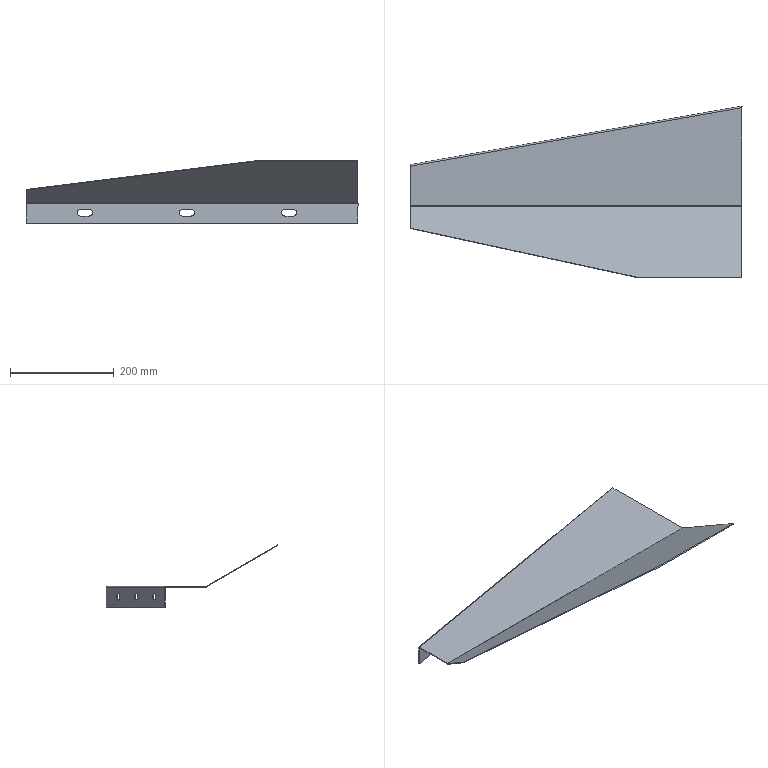Part | SolidWorks | features BaseBody 1 | 1 solid | 34 faces | box 640.37 x 331.413 x 119.799 mm | volume 282852 mm3 | plane 19 | cylinder 13 | spline 2 | commonest cylinder face diameters 13 x9 3 x2 6 x2
STEP:
#1=CARTESIAN_POINT('',(201.948,132.034,-18.5));
#2=VERTEX_POINT('',#1);
#3=CARTESIAN_POINT('',(195.547,130.905,-12.));
#4=VERTEX_POINT('',#3);
#5=CARTESIAN_POINT('',(195.547,130.905,-18.5));
#6=DIRECTION('',(0.1736,-0.9848,0.));
#7=DIRECTION('',(0.9848,0.1736,0.));
#8=AXIS2_PLACEMENT_3D('',#5,#6,#7);
#9=CIRCLE('',#8,6.5);
#10=EDGE_CURVE('',#2,#4,#9,.T.);
#11=ORIENTED_EDGE('',*,*,#10,.F.);
#12=CARTESIAN_POINT('',(202.209,130.556,-18.5));
#13=VERTEX_POINT('',#12);
#14=CARTESIAN_POINT('',(201.948,132.034,-18.5));
#15=DIRECTION('',(0.1736,-0.9848,0.));
#16=VECTOR('',#15,1000.);
#17=LINE('',#14,#16);
#18=EDGE_CURVE('',#2,#13,#17,.T.);
#19=ORIENTED_EDGE('',*,*,#18,.T.);
#20=CARTESIAN_POINT('',(195.807,129.428,-12.));
#21=VERTEX_POINT('',#20);
#22=CARTESIAN_POINT('',(195.807,129.428,-18.5));
#23=DIRECTION('',(-0.1736,0.9848,0.));
#24=DIRECTION('',(0.9848,0.1736,0.));
#25=AXIS2_PLACEMENT_3D('',#22,#23,#24);
#26=CIRCLE('',#25,6.5);
#27=EDGE_CURVE('',#21,#13,#26,.T.);
#28=ORIENTED_EDGE('',*,*,#27,.F.);
#29=CARTESIAN_POINT('',(195.807,129.428,-12.));
#30=DIRECTION('',(-0.1736,0.9848,0.));
#31=VECTOR('',#30,1000.);
#32=LINE('',#29,#31);
#33=EDGE_CURVE('',#21,#4,#32,.T.);
#34=ORIENTED_EDGE('',*,*,#33,.T.);
#35=EDGE_LOOP('',(#11,#19,#28,#34));
#36=FACE_OUTER_BOUND('',#35,.T.);
#37=CARTESIAN_POINT('',(195.547,130.905,-18.5));
#38=DIRECTION('',(0.1736,-0.9848,0.));
#39=DIRECTION('',(0.9848,0.1736,0.));
#40=AXIS2_PLACEMENT_3D('',#37,#38,#39);
#41=CYLINDRICAL_SURFACE('',#40,6.5);
#42=ADVANCED_FACE('',(#36),#41,.F.);
#43=CARTESIAN_POINT('',(-191.975,62.574,-18.5));
#44=VERTEX_POINT('',#43);
#45=CARTESIAN_POINT('',(-198.376,61.446,-12.));
#46=VERTEX_POINT('',#45);
#47=CARTESIAN_POINT('',(-198.376,61.446,-18.5));
#48=DIRECTION('',(0.1736,-0.9848,0.));
#49=DIRECTION('',(0.9848,0.1736,0.));
#50=AXIS2_PLACEMENT_3D('',#47,#48,#49);
#51=CIRCLE('',#50,6.5);
#52=EDGE_CURVE('',#44,#46,#51,.T.);
#53=ORIENTED_EDGE('',*,*,#52,.F.);
#54=CARTESIAN_POINT('',(-191.715,61.097,-18.5));
#55=VERTEX_POINT('',#54);
#56=CARTESIAN_POINT('',(-191.975,62.574,-18.5));
#57=DIRECTION('',(0.1736,-0.9848,0.));
#58=VECTOR('',#57,1000.);
#59=LINE('',#56,#58);
#60=EDGE_CURVE('',#44,#55,#59,.T.);
#61=ORIENTED_EDGE('',*,*,#60,.T.);
#62=CARTESIAN_POINT('',(-198.116,59.968,-12.));
#63=VERTEX_POINT('',#62);
#64=CARTESIAN_POINT('',(-198.116,59.968,-18.5));
#65=DIRECTION('',(-0.1736,0.9848,0.));
#66=DIRECTION('',(0.9848,0.1736,0.));
#67=AXIS2_PLACEMENT_3D('',#64,#65,#66);
#68=CIRCLE('',#67,6.5);
#69=EDGE_CURVE('',#63,#55,#68,.T.);
#70=ORIENTED_EDGE('',*,*,#69,.F.);
#71=CARTESIAN_POINT('',(-198.116,59.968,-12.));
#72=DIRECTION('',(-0.1736,0.9848,0.));
#73=VECTOR('',#72,1000.);
#74=LINE('',#71,#73);
#75=EDGE_CURVE('',#63,#46,#74,.T.);
#76=ORIENTED_EDGE('',*,*,#75,.T.);
#77=EDGE_LOOP('',(#53,#61,#70,#76));
#78=FACE_OUTER_BOUND('',#77,.T.);
#79=CARTESIAN_POINT('',(-198.376,61.446,-18.5));
#80=DIRECTION('',(0.1736,-0.9848,0.));
#81=DIRECTION('',(0.9848,0.1736,0.));
#82=AXIS2_PLACEMENT_3D('',#79,#80,#81);
#83=CYLINDRICAL_SURFACE('',#82,6.5);
#84=ADVANCED_FACE('',(#78),#83,.F.);
#85=CARTESIAN_POINT('',(4.987,97.304,-18.5));
#86=VERTEX_POINT('',#85);
#87=CARTESIAN_POINT('',(-1.415,96.175,-12.));
#88=VERTEX_POINT('',#87);
#89=CARTESIAN_POINT('',(-1.415,96.175,-18.5));
#90=DIRECTION('',(0.1736,-0.9848,0.));
#91=DIRECTION('',(0.9848,0.1736,0.));
#92=AXIS2_PLACEMENT_3D('',#89,#90,#91);
#93=CIRCLE('',#92,6.5);
#94=EDGE_CURVE('',#86,#88,#93,.T.);
#95=ORIENTED_EDGE('',*,*,#94,.F.);
#96=CARTESIAN_POINT('',(5.247,95.827,-18.5));
#97=VERTEX_POINT('',#96);
#98=CARTESIAN_POINT('',(4.987,97.304,-18.5));
#99=DIRECTION('',(0.1736,-0.9848,0.));
#100=VECTOR('',#99,1000.);
#101=LINE('',#98,#100);
#102=EDGE_CURVE('',#86,#97,#101,.T.);
#103=ORIENTED_EDGE('',*,*,#102,.T.);
#104=CARTESIAN_POINT('',(-1.154,94.698,-12.));
#105=VERTEX_POINT('',#104);
#106=CARTESIAN_POINT('',(-1.154,94.698,-18.5));
#107=DIRECTION('',(-0.1736,0.9848,0.));
#108=DIRECTION('',(0.9848,0.1736,0.));
#109=AXIS2_PLACEMENT_3D('',#106,#107,#108);
#110=CIRCLE('',#109,6.5);
#111=EDGE_CURVE('',#105,#97,#110,.T.);
#112=ORIENTED_EDGE('',*,*,#111,.F.);
#113=CARTESIAN_POINT('',(-1.154,94.698,-12.));
#114=DIRECTION('',(-0.1736,0.9848,0.));
#115=VECTOR('',#114,1000.);
#116=LINE('',#113,#115);
#117=EDGE_CURVE('',#105,#88,#116,.T.);
#118=ORIENTED_EDGE('',*,*,#117,.T.);
#119=EDGE_LOOP('',(#95,#103,#112,#118));
#120=FACE_OUTER_BOUND('',#119,.T.);
#121=CARTESIAN_POINT('',(-1.415,96.175,-18.5));
#122=DIRECTION('',(0.1736,-0.9848,0.));
#123=DIRECTION('',(0.9848,0.1736,0.));
#124=AXIS2_PLACEMENT_3D('',#121,#122,#123);
#125=CYLINDRICAL_SURFACE('',#124,6.5);
#126=ADVANCED_FACE('',(#120),#125,.F.);
#127=CARTESIAN_POINT('',(320.,149.803,1.5));
#128=VERTEX_POINT('',#127);
#129=CARTESIAN_POINT('',(-320.,36.954,1.5));
#130=VERTEX_POINT('',#129);
#131=CARTESIAN_POINT('',(320.,149.803,1.5));
#132=DIRECTION('',(-0.9848,-0.1736,0.));
#133=VECTOR('',#132,1000.);
#134=LINE('',#131,#133);
#135=EDGE_CURVE('',#128,#130,#134,.T.);
#136=ORIENTED_EDGE('',*,*,#135,.T.);
#137=CARTESIAN_POINT('',(-320.,-39.196,1.5));
#138=VERTEX_POINT('',#137);
#139=CARTESIAN_POINT('',(-320.,30.681,1.5));
#140=DIRECTION('',(0.,-1.,0.));
#141=VECTOR('',#140,1000.);
#142=LINE('',#139,#141);
#143=EDGE_CURVE('',#130,#138,#142,.T.);
#144=ORIENTED_EDGE('',*,*,#143,.T.);
#145=CARTESIAN_POINT('',(320.,-39.196,1.5));
#146=VERTEX_POINT('',#145);
#147=CARTESIAN_POINT('',(23.108,-39.196,1.5));
#148=DIRECTION('',(1.,0.,0.));
#149=VECTOR('',#148,1000.);
#150=LINE('',#147,#149);
#151=EDGE_CURVE('',#138,#146,#150,.T.);
#152=ORIENTED_EDGE('',*,*,#151,.T.);
#153=CARTESIAN_POINT('',(320.,30.681,1.5));
#154=DIRECTION('',(0.,1.,0.));
#155=VECTOR('',#154,1000.);
#156=LINE('',#153,#155);
#157=EDGE_CURVE('',#146,#128,#156,.T.);
#158=ORIENTED_EDGE('',*,*,#157,.T.);
#159=EDGE_LOOP('',(#136,#144,#152,#158));
#160=FACE_OUTER_BOUND('',#159,.T.);
#161=CARTESIAN_POINT('',(23.108,30.681,1.5));
#162=DIRECTION('',(0.,0.,1.));
#163=DIRECTION('',(1.,0.,0.));
#164=AXIS2_PLACEMENT_3D('',#161,#162,#163);
#165=PLANE('',#164);
#166=ADVANCED_FACE('',(#160),#165,.T.);
#167=CARTESIAN_POINT('',(-320.,36.954,0.));
#168=VERTEX_POINT('',#167);
#169=CARTESIAN_POINT('',(-320.,36.954,0.75));
#170=DIRECTION('',(0.,0.,1.));
#171=VECTOR('',#170,1000.);
#172=LINE('',#169,#171);
#173=EDGE_CURVE('',#168,#130,#172,.T.);
#174=ORIENTED_EDGE('',*,*,#173,.F.);
#175=CARTESIAN_POINT('',(-320.,-39.196,0.));
#176=VERTEX_POINT('',#175);
#177=CARTESIAN_POINT('',(-320.,-40.,0.));
#178=DIRECTION('',(0.,-1.,0.));
#179=VECTOR('',#178,1000.);
#180=LINE('',#177,#179);
#181=EDGE_CURVE('',#168,#176,#180,.T.);
#182=ORIENTED_EDGE('',*,*,#181,.T.);
#183=CARTESIAN_POINT('',(-320.,-40.696,0.4019));
#184=VERTEX_POINT('',#183);
#185=CARTESIAN_POINT('',(-320.,-39.196,3.));
#186=DIRECTION('',(-1.,0.,0.));
#187=DIRECTION('',(0.,-1.,0.));
#188=AXIS2_PLACEMENT_3D('',#185,#186,#187);
#189=CIRCLE('',#188,3.);
#190=EDGE_CURVE('',#176,#184,#189,.T.);
#191=ORIENTED_EDGE('',*,*,#190,.T.);
#192=CARTESIAN_POINT('',(-320.,-83.301,25.));
#193=VERTEX_POINT('',#192);
#194=CARTESIAN_POINT('',(-320.,-40.696,0.4019));
#195=DIRECTION('',(0.,-0.866,0.5));
#196=VECTOR('',#195,1000.);
#197=LINE('',#194,#196);
#198=EDGE_CURVE('',#184,#193,#197,.T.);
#199=ORIENTED_EDGE('',*,*,#198,.T.);
#200=CARTESIAN_POINT('',(-320.,-82.551,26.299));
#201=VERTEX_POINT('',#200);
#202=CARTESIAN_POINT('',(-320.,-83.301,25.));
#203=DIRECTION('',(0.,0.5,0.866));
#204=VECTOR('',#203,1000.);
#205=LINE('',#202,#204);
#206=EDGE_CURVE('',#193,#201,#205,.T.);
#207=ORIENTED_EDGE('',*,*,#206,.T.);
#208=CARTESIAN_POINT('',(-320.,-39.946,1.701));
#209=VERTEX_POINT('',#208);
#210=CARTESIAN_POINT('',(-320.,-108.39,41.217));
#211=DIRECTION('',(0.,-0.866,0.5));
#212=VECTOR('',#211,1000.);
#213=LINE('',#210,#212);
#214=EDGE_CURVE('',#209,#201,#213,.T.);
#215=ORIENTED_EDGE('',*,*,#214,.F.);
#216=CARTESIAN_POINT('',(-320.,-39.196,3.));
#217=DIRECTION('',(1.,0.,0.));
#218=DIRECTION('',(0.,-1.,0.));
#219=AXIS2_PLACEMENT_3D('',#216,#217,#218);
#220=CIRCLE('',#219,1.5);
#221=EDGE_CURVE('',#209,#138,#220,.T.);
#222=ORIENTED_EDGE('',*,*,#221,.T.);
#223=ORIENTED_EDGE('',*,*,#143,.F.);
#224=EDGE_LOOP('',(#174,#182,#191,#199,#207,#215,#222,#223));
#225=FACE_OUTER_BOUND('',#224,.T.);
#226=CARTESIAN_POINT('',(-320.,-40.,0.));
#227=DIRECTION('',(-1.,0.,0.));
#228=DIRECTION('',(0.,-1.,0.));
#229=AXIS2_PLACEMENT_3D('',#226,#227,#228);
#230=PLANE('',#229);
#231=ADVANCED_FACE('',(#225),#230,.T.);
#232=ORIENTED_EDGE('',*,*,#135,.F.);
#233=CARTESIAN_POINT('',(320.,152.849,-1.5));
#234=VERTEX_POINT('',#233);
#235=CARTESIAN_POINT('',(320.,149.803,1.5));
#236=CARTESIAN_POINT('',(319.988,150.002,1.5));
#237=CARTESIAN_POINT('',(319.975,150.198,1.481));
#238=CARTESIAN_POINT('',(319.952,150.585,1.404));
#239=CARTESIAN_POINT('',(319.94,150.777,1.346));
#240=CARTESIAN_POINT('',(319.921,151.14,1.196));
#241=CARTESIAN_POINT('',(319.912,151.314,1.104));
#242=CARTESIAN_POINT('',(319.899,151.644,0.8849));
#243=CARTESIAN_POINT('',(319.894,151.798,0.7594));
#244=CARTESIAN_POINT('',(319.89,152.078,0.4833));
#245=CARTESIAN_POINT('',(319.89,152.205,0.3309));
#246=CARTESIAN_POINT('',(319.895,152.429,0.002871));
#247=CARTESIAN_POINT('',(319.901,152.523,-0.1695));
#248=CARTESIAN_POINT('',(319.918,152.678,-0.5306));
#249=CARTESIAN_POINT('',(319.93,152.739,-0.7211));
#250=CARTESIAN_POINT('',(319.96,152.822,-1.107));
#251=CARTESIAN_POINT('',(319.978,152.845,-1.302));
#252=CARTESIAN_POINT('',(320.,152.849,-1.5));
#253=B_SPLINE_CURVE_WITH_KNOTS('',3,(#235,#236,#237,#238,#239,#240,#241,#242,#243,#244,#245,#246,#247,#248,#249,#250,#251,#252),.UNSPECIFIED.,.F.,.F.,(4,2,2,2,2,2,2,2,4),(0.,0.000592,0.001184,0.001776,0.002368,0.00296,0.003552,0.004144,0.004736),.UNSPECIFIED.);
#254=EDGE_CURVE('',#128,#234,#253,.T.);
#255=ORIENTED_EDGE('',*,*,#254,.T.);
#256=CARTESIAN_POINT('',(-320.,40.,-1.5));
#257=VERTEX_POINT('',#256);
#258=CARTESIAN_POINT('',(-0.5209,96.333,-1.5));
#259=DIRECTION('',(-0.9848,-0.1736,0.));
#260=VECTOR('',#259,1000.);
#261=LINE('',#258,#260);
#262=EDGE_CURVE('',#234,#257,#261,.T.);
#263=ORIENTED_EDGE('',*,*,#262,.T.);
#264=CARTESIAN_POINT('',(-320.,40.,-1.5));
#265=CARTESIAN_POINT('',(-320.022,39.996,-1.302));
#266=CARTESIAN_POINT('',(-320.04,39.973,-1.107));
#267=CARTESIAN_POINT('',(-320.07,39.89,-0.7214));
#268=CARTESIAN_POINT('',(-320.082,39.829,-0.5307));
#269=CARTESIAN_POINT('',(-320.099,39.674,-0.1696));
#270=CARTESIAN_POINT('',(-320.105,39.579,0.002791));
#271=CARTESIAN_POINT('',(-320.11,39.356,0.3306));
#272=CARTESIAN_POINT('',(-320.11,39.229,0.4833));
#273=CARTESIAN_POINT('',(-320.106,38.949,0.7593));
#274=CARTESIAN_POINT('',(-320.101,38.795,0.8847));
#275=CARTESIAN_POINT('',(-320.088,38.464,1.104));
#276=CARTESIAN_POINT('',(-320.079,38.291,1.196));
#277=CARTESIAN_POINT('',(-320.06,37.928,1.346));
#278=CARTESIAN_POINT('',(-320.048,37.736,1.404));
#279=CARTESIAN_POINT('',(-320.025,37.349,1.481));
#280=CARTESIAN_POINT('',(-320.012,37.153,1.5));
#281=CARTESIAN_POINT('',(-320.,36.954,1.5));
#282=B_SPLINE_CURVE_WITH_KNOTS('',3,(#264,#265,#266,#267,#268,#269,#270,#271,#272,#273,#274,#275,#276,#277,#278,#279,#280,#281),.UNSPECIFIED.,.F.,.F.,(4,2,2,2,2,2,2,2,4),(0.,0.000592,0.001184,0.001776,0.002368,0.00296,0.003552,0.004144,0.004736),.UNSPECIFIED.);
#283=EDGE_CURVE('',#257,#130,#282,.T.);
#284=ORIENTED_EDGE('',*,*,#283,.T.);
#285=EDGE_LOOP('',(#232,#255,#263,#284));
#286=FACE_OUTER_BOUND('',#285,.T.);
#287=CARTESIAN_POINT('',(0.,93.378,-1.5));
#288=DIRECTION('',(-0.9848,-0.1736,0.));
#289=DIRECTION('',(0.1736,-0.9848,0.));
#290=AXIS2_PLACEMENT_3D('',#287,#288,#289);
#291=CYLINDRICAL_SURFACE('',#290,3.);
#292=ADVANCED_FACE('',(#286),#291,.T.);
#293=CARTESIAN_POINT('',(320.,149.803,0.));
#294=VERTEX_POINT('',#293);
#295=CARTESIAN_POINT('',(320.,149.803,0.));
#296=DIRECTION('',(0.,0.,1.));
#297=VECTOR('',#296,1000.);
#298=LINE('',#295,#297);
#299=EDGE_CURVE('',#294,#128,#298,.T.);
#300=ORIENTED_EDGE('',*,*,#299,.T.);
#301=ORIENTED_EDGE('',*,*,#157,.F.);
#302=CARTESIAN_POINT('',(320.,-39.946,1.701));
#303=VERTEX_POINT('',#302);
#304=CARTESIAN_POINT('',(320.,-39.196,3.));
#305=DIRECTION('',(-1.,0.,0.));
#306=DIRECTION('',(0.,-1.,0.));
#307=AXIS2_PLACEMENT_3D('',#304,#305,#306);
#308=CIRCLE('',#307,1.5);
#309=EDGE_CURVE('',#146,#303,#308,.T.);
#310=ORIENTED_EDGE('',*,*,#309,.T.);
#311=CARTESIAN_POINT('',(320.,-177.814,81.299));
#312=VERTEX_POINT('',#311);
#313=CARTESIAN_POINT('',(320.,-108.39,41.217));
#314=DIRECTION('',(0.,0.866,-0.5));
#315=VECTOR('',#314,1000.);
#316=LINE('',#313,#315);
#317=EDGE_CURVE('',#312,#303,#316,.T.);
#318=ORIENTED_EDGE('',*,*,#317,.F.);
#319=CARTESIAN_POINT('',(320.,-178.564,80.));
#320=VERTEX_POINT('',#319);
#321=CARTESIAN_POINT('',(320.,-177.814,81.299));
#322=DIRECTION('',(0.,-0.5,-0.866));
#323=VECTOR('',#322,1000.);
#324=LINE('',#321,#323);
#325=EDGE_CURVE('',#312,#320,#324,.T.);
#326=ORIENTED_EDGE('',*,*,#325,.T.);
#327=CARTESIAN_POINT('',(320.,-40.696,0.4019));
#328=VERTEX_POINT('',#327);
#329=CARTESIAN_POINT('',(320.,-178.564,80.));
#330=DIRECTION('',(0.,0.866,-0.5));
#331=VECTOR('',#330,1000.);
#332=LINE('',#329,#331);
#333=EDGE_CURVE('',#320,#328,#332,.T.);
#334=ORIENTED_EDGE('',*,*,#333,.T.);
#335=CARTESIAN_POINT('',(320.,-39.196,0.));
#336=VERTEX_POINT('',#335);
#337=CARTESIAN_POINT('',(320.,-39.196,3.));
#338=DIRECTION('',(1.,0.,0.));
#339=DIRECTION('',(0.,-1.,0.));
#340=AXIS2_PLACEMENT_3D('',#337,#338,#339);
#341=CIRCLE('',#340,3.);
#342=EDGE_CURVE('',#328,#336,#341,.T.);
#343=ORIENTED_EDGE('',*,*,#342,.T.);
#344=CARTESIAN_POINT('',(320.,40.,0.));
#345=DIRECTION('',(0.,1.,0.));
#346=VECTOR('',#345,1000.);
#347=LINE('',#344,#346);
#348=EDGE_CURVE('',#336,#294,#347,.T.);
#349=ORIENTED_EDGE('',*,*,#348,.T.);
#350=EDGE_LOOP('',(#300,#301,#310,#318,#326,#334,#343,#349));
#351=FACE_OUTER_BOUND('',#350,.T.);
#352=CARTESIAN_POINT('',(320.,40.,0.));
#353=DIRECTION('',(1.,0.,0.));
#354=DIRECTION('',(0.,0.,-1.));
#355=AXIS2_PLACEMENT_3D('',#352,#353,#354);
#356=PLANE('',#355);
#357=ADVANCED_FACE('',(#351),#356,.T.);
#358=ORIENTED_EDGE('',*,*,#309,.F.);
#359=ORIENTED_EDGE('',*,*,#151,.F.);
#360=ORIENTED_EDGE('',*,*,#221,.F.);
#361=CARTESIAN_POINT('',(0.,-39.946,1.701));
#362=DIRECTION('',(-1.,0.,0.));
#363=VECTOR('',#362,1000.);
#364=LINE('',#361,#363);
#365=EDGE_CURVE('',#303,#209,#364,.T.);
#366=ORIENTED_EDGE('',*,*,#365,.F.);
#367=EDGE_LOOP('',(#358,#359,#360,#366));
#368=FACE_OUTER_BOUND('',#367,.T.);
#369=CARTESIAN_POINT('',(0.,-39.196,3.));
#370=DIRECTION('',(-1.,0.,0.));
#371=DIRECTION('',(0.,-1.,0.));
#372=AXIS2_PLACEMENT_3D('',#369,#370,#371);
#373=CYLINDRICAL_SURFACE('',#372,1.5);
#374=ADVANCED_FACE('',(#368),#373,.F.);
#375=ORIENTED_EDGE('',*,*,#181,.F.);
#376=CARTESIAN_POINT('',(320.,149.803,0.));
#377=DIRECTION('',(-0.9848,-0.1736,0.));
#378=VECTOR('',#377,1000.);
#379=LINE('',#376,#378);
#380=EDGE_CURVE('',#294,#168,#379,.T.);
#381=ORIENTED_EDGE('',*,*,#380,.F.);
#382=ORIENTED_EDGE('',*,*,#348,.F.);
#383=CARTESIAN_POINT('',(23.108,-39.196,0.));
#384=DIRECTION('',(1.,0.,0.));
#385=VECTOR('',#384,1000.);
#386=LINE('',#383,#385);
#387=EDGE_CURVE('',#176,#336,#386,.T.);
#388=ORIENTED_EDGE('',*,*,#387,.F.);
#389=EDGE_LOOP('',(#375,#381,#382,#388));
#390=FACE_OUTER_BOUND('',#389,.T.);
#391=CARTESIAN_POINT('',(23.108,30.681,0.));
#392=DIRECTION('',(0.,0.,1.));
#393=DIRECTION('',(1.,0.,0.));
#394=AXIS2_PLACEMENT_3D('',#391,#392,#393);
#395=PLANE('',#394);
#396=ADVANCED_FACE('',(#390),#395,.F.);
#397=CARTESIAN_POINT('',(320.26,151.372,-1.5));
#398=VERTEX_POINT('',#397);
#399=CARTESIAN_POINT('',(320.,149.803,0.));
#400=CARTESIAN_POINT('',(320.009,150.006,0.));
#401=CARTESIAN_POINT('',(320.019,150.205,-0.03888));
#402=CARTESIAN_POINT('',(320.036,150.485,-0.1518));
#403=CARTESIAN_POINT('',(320.043,150.573,-0.1979));
#404=CARTESIAN_POINT('',(320.058,150.741,-0.3065));
#405=CARTESIAN_POINT('',(320.067,150.821,-0.3698));
#406=CARTESIAN_POINT('',(320.086,150.965,-0.5082));
#407=CARTESIAN_POINT('',(320.097,151.03,-0.5836));
#408=CARTESIAN_POINT('',(320.121,151.145,-0.7469));
#409=CARTESIAN_POINT('',(320.135,151.195,-0.8347));
#410=CARTESIAN_POINT('',(320.18,151.318,-1.105));
#411=CARTESIAN_POINT('',(320.217,151.364,-1.302));
#412=CARTESIAN_POINT('',(320.26,151.372,-1.5));
#413=B_SPLINE_CURVE_WITH_KNOTS('',3,(#399,#400,#401,#402,#403,#404,#405,#406,#407,#408,#409,#410,#411,#412),.UNSPECIFIED.,.F.,.F.,(4,2,2,2,2,2,4),(0.,0.0006004,0.0009005,0.001201,0.001501,0.001801,0.002401),.UNSPECIFIED.);
#414=EDGE_CURVE('',#294,#398,#413,.T.);
#415=ORIENTED_EDGE('',*,*,#414,.T.);
#416=CARTESIAN_POINT('',(320.26,151.372,-1.5));
#417=DIRECTION('',(0.1736,-0.9848,0.));
#418=VECTOR('',#417,1000.);
#419=LINE('',#416,#418);
#420=EDGE_CURVE('',#234,#398,#419,.T.);
#421=ORIENTED_EDGE('',*,*,#420,.F.);
#422=ORIENTED_EDGE('',*,*,#254,.F.);
#423=ORIENTED_EDGE('',*,*,#299,.F.);
#424=EDGE_LOOP('',(#415,#421,#422,#423));
#425=FACE_OUTER_BOUND('',#424,.T.);
#426=CARTESIAN_POINT('',(320.,149.803,1.516));
#427=CARTESIAN_POINT('',(319.957,150.483,1.516));
#428=CARTESIAN_POINT('',(319.856,152.07,0.9637));
#429=CARTESIAN_POINT('',(319.898,152.847,-0.5977));
#430=CARTESIAN_POINT('',(319.997,152.865,-1.5));
#431=CARTESIAN_POINT('',(320.,149.803,1.511));
#432=CARTESIAN_POINT('',(319.957,150.481,1.511));
#433=CARTESIAN_POINT('',(319.857,152.066,0.9594));
#434=CARTESIAN_POINT('',(319.899,152.842,-0.5993));
#435=CARTESIAN_POINT('',(319.998,152.86,-1.5));
#436=CARTESIAN_POINT('',(320.,149.803,1.505));
#437=CARTESIAN_POINT('',(319.957,150.48,1.505));
#438=CARTESIAN_POINT('',(319.857,152.062,0.9551));
#439=CARTESIAN_POINT('',(319.9,152.837,-0.6008));
#440=CARTESIAN_POINT('',(319.999,152.854,-1.5));
#441=CARTESIAN_POINT('',(320.,149.803,1.5));
#442=CARTESIAN_POINT('',(319.958,150.479,1.5));
#443=CARTESIAN_POINT('',(319.858,152.059,0.9508));
#444=CARTESIAN_POINT('',(319.901,152.832,-0.6024));
#445=CARTESIAN_POINT('',(320.,152.849,-1.5));
#446=CARTESIAN_POINT('',(320.,149.803,1.));
#447=CARTESIAN_POINT('',(319.977,150.369,1.));
#448=CARTESIAN_POINT('',(319.923,151.69,0.5423));
#449=CARTESIAN_POINT('',(319.988,152.339,-0.752));
#450=CARTESIAN_POINT('',(320.087,152.357,-1.5));
#451=CARTESIAN_POINT('',(320.,149.803,0.5));
#452=CARTESIAN_POINT('',(319.996,150.258,0.5));
#453=CARTESIAN_POINT('',(319.988,151.321,0.1339));
#454=CARTESIAN_POINT('',(320.074,151.847,-0.9016));
#455=CARTESIAN_POINT('',(320.174,151.864,-1.5));
#456=CARTESIAN_POINT('',(320.,149.803,0.));
#457=CARTESIAN_POINT('',(320.016,150.148,0.));
#458=CARTESIAN_POINT('',(320.053,150.953,-0.2746));
#459=CARTESIAN_POINT('',(320.161,151.355,-1.051));
#460=CARTESIAN_POINT('',(320.26,151.372,-1.5));
#461=CARTESIAN_POINT('',(320.,149.803,-0.005053));
#462=CARTESIAN_POINT('',(320.016,150.146,-0.005053));
#463=CARTESIAN_POINT('',(320.054,150.949,-0.2787));
#464=CARTESIAN_POINT('',(320.162,151.35,-1.053));
#465=CARTESIAN_POINT('',(320.261,151.367,-1.5));
#466=CARTESIAN_POINT('',(320.,149.803,-0.01011));
#467=CARTESIAN_POINT('',(320.016,150.145,-0.01011));
#468=CARTESIAN_POINT('',(320.054,150.945,-0.2829));
#469=CARTESIAN_POINT('',(320.163,151.345,-1.054));
#470=CARTESIAN_POINT('',(320.262,151.362,-1.5));
#471=CARTESIAN_POINT('',(320.,149.803,-0.01516));
#472=CARTESIAN_POINT('',(320.017,150.144,-0.01516));
#473=CARTESIAN_POINT('',(320.055,150.941,-0.287));
#474=CARTESIAN_POINT('',(320.164,151.34,-1.056));
#475=CARTESIAN_POINT('',(320.263,151.357,-1.5));
#476=B_SPLINE_SURFACE_WITH_KNOTS('',3,3,((#426,#427,#428,#429,#430),(#431,#432,#433,#434,#435),(#436,#437,#438,#439,#440),(#441,#442,#443,#444,#445),(#446,#447,#448,#449,#450),(#451,#452,#453,#454,#455),(#456,#457,#458,#459,#460),(#461,#462,#463,#464,#465),(#466,#467,#468,#469,#470),(#471,#472,#473,#474,#475)),.UNSPECIFIED.,.F.,.F.,.F.,(4,3,3,4),(4,1,4),(-0.1516,-0.15,0.,0.001516),(-0.3434,-0.1962,0.),.UNSPECIFIED.);
#477=ADVANCED_FACE('',(#425),#476,.T.);
#478=CARTESIAN_POINT('',(-319.74,38.523,-1.5));
#479=VERTEX_POINT('',#478);
#480=CARTESIAN_POINT('',(-319.74,38.523,-1.5));
#481=CARTESIAN_POINT('',(-319.783,38.515,-1.302));
#482=CARTESIAN_POINT('',(-319.82,38.469,-1.108));
#483=CARTESIAN_POINT('',(-319.865,38.346,-0.8351));
#484=CARTESIAN_POINT('',(-319.879,38.297,-0.749));
#485=CARTESIAN_POINT('',(-319.903,38.183,-0.5862));
#486=CARTESIAN_POINT('',(-319.914,38.117,-0.5089));
#487=CARTESIAN_POINT('',(-319.933,37.973,-0.3704));
#488=CARTESIAN_POINT('',(-319.942,37.894,-0.3084));
#489=CARTESIAN_POINT('',(-319.957,37.726,-0.199));
#490=CARTESIAN_POINT('',(-319.964,37.636,-0.1521));
#491=CARTESIAN_POINT('',(-319.981,37.358,-0.03974));
#492=CARTESIAN_POINT('',(-319.991,37.157,0.));
#493=CARTESIAN_POINT('',(-320.,36.954,0.));
#494=B_SPLINE_CURVE_WITH_KNOTS('',3,(#480,#481,#482,#483,#484,#485,#486,#487,#488,#489,#490,#491,#492,#493),.UNSPECIFIED.,.F.,.F.,(4,2,2,2,2,2,4),(0.,0.0006004,0.0009006,0.001201,0.001501,0.001801,0.002401),.UNSPECIFIED.);
#495=EDGE_CURVE('',#479,#168,#494,.T.);
#496=ORIENTED_EDGE('',*,*,#495,.T.);
#497=ORIENTED_EDGE('',*,*,#173,.T.);
#498=ORIENTED_EDGE('',*,*,#283,.F.);
#499=CARTESIAN_POINT('',(-319.74,38.523,-1.5));
#500=DIRECTION('',(-0.1736,0.9848,0.));
#501=VECTOR('',#500,1000.);
#502=LINE('',#499,#501);
#503=EDGE_CURVE('',#479,#257,#502,.T.);
#504=ORIENTED_EDGE('',*,*,#503,.F.);
#505=EDGE_LOOP('',(#496,#497,#498,#504));
#506=FACE_OUTER_BOUND('',#505,.T.);
#507=CARTESIAN_POINT('',(-320.,36.954,-0.01516));
#508=CARTESIAN_POINT('',(-319.983,37.295,-0.01516));
#509=CARTESIAN_POINT('',(-319.945,38.092,-0.287));
#510=CARTESIAN_POINT('',(-319.836,38.49,-1.056));
#511=CARTESIAN_POINT('',(-319.737,38.508,-1.5));
#512=CARTESIAN_POINT('',(-320.,36.954,-0.0101));
#513=CARTESIAN_POINT('',(-319.984,37.296,-0.0101));
#514=CARTESIAN_POINT('',(-319.946,38.096,-0.2828));
#515=CARTESIAN_POINT('',(-319.837,38.495,-1.054));
#516=CARTESIAN_POINT('',(-319.738,38.513,-1.5));
#517=CARTESIAN_POINT('',(-320.,36.954,-0.005052));
#518=CARTESIAN_POINT('',(-319.984,37.297,-0.005052));
#519=CARTESIAN_POINT('',(-319.946,38.1,-0.2787));
#520=CARTESIAN_POINT('',(-319.838,38.5,-1.053));
#521=CARTESIAN_POINT('',(-319.739,38.518,-1.5));
#522=CARTESIAN_POINT('',(-320.,36.954,0.));
#523=CARTESIAN_POINT('',(-319.984,37.298,0.));
#524=CARTESIAN_POINT('',(-319.947,38.103,-0.2746));
#525=CARTESIAN_POINT('',(-319.839,38.505,-1.051));
#526=CARTESIAN_POINT('',(-319.74,38.523,-1.5));
#527=CARTESIAN_POINT('',(-320.,36.954,0.5));
#528=CARTESIAN_POINT('',(-320.004,37.409,0.5));
#529=CARTESIAN_POINT('',(-320.012,38.472,0.1339));
#530=CARTESIAN_POINT('',(-319.926,38.998,-0.9016));
#531=CARTESIAN_POINT('',(-319.826,39.015,-1.5));
#532=CARTESIAN_POINT('',(-320.,36.954,1.));
#533=CARTESIAN_POINT('',(-320.023,37.519,1.));
#534=CARTESIAN_POINT('',(-320.077,38.841,0.5423));
#535=CARTESIAN_POINT('',(-320.012,39.49,-0.752));
#536=CARTESIAN_POINT('',(-319.913,39.508,-1.5));
#537=CARTESIAN_POINT('',(-320.,36.954,1.5));
#538=CARTESIAN_POINT('',(-320.042,37.63,1.5));
#539=CARTESIAN_POINT('',(-320.142,39.209,0.9508));
#540=CARTESIAN_POINT('',(-320.099,39.983,-0.6024));
#541=CARTESIAN_POINT('',(-320.,40.,-1.5));
#542=CARTESIAN_POINT('',(-320.,36.954,1.505));
#543=CARTESIAN_POINT('',(-320.043,37.631,1.505));
#544=CARTESIAN_POINT('',(-320.143,39.213,0.9551));
#545=CARTESIAN_POINT('',(-320.1,39.988,-0.6008));
#546=CARTESIAN_POINT('',(-320.001,40.005,-1.5));
#547=CARTESIAN_POINT('',(-320.,36.954,1.51));
#548=CARTESIAN_POINT('',(-320.043,37.632,1.51));
#549=CARTESIAN_POINT('',(-320.143,39.217,0.9594));
#550=CARTESIAN_POINT('',(-320.101,39.993,-0.5993));
#551=CARTESIAN_POINT('',(-320.002,40.01,-1.5));
#552=CARTESIAN_POINT('',(-320.,36.954,1.516));
#553=CARTESIAN_POINT('',(-320.043,37.633,1.516));
#554=CARTESIAN_POINT('',(-320.144,39.221,0.9637));
#555=CARTESIAN_POINT('',(-320.102,39.998,-0.5977));
#556=CARTESIAN_POINT('',(-320.003,40.016,-1.5));
#557=B_SPLINE_SURFACE_WITH_KNOTS('',3,3,((#507,#508,#509,#510,#511),(#512,#513,#514,#515,#516),(#517,#518,#519,#520,#521),(#522,#523,#524,#525,#526),(#527,#528,#529,#530,#531),(#532,#533,#534,#535,#536),(#537,#538,#539,#540,#541),(#542,#543,#544,#545,#546),(#547,#548,#549,#550,#551),(#552,#553,#554,#555,#556)),.UNSPECIFIED.,.F.,.F.,.F.,(4,3,3,4),(4,1,4),(-0.001516,0.,0.15,0.1516),(0.,0.1472,0.3434),.UNSPECIFIED.);
#558=ADVANCED_FACE('',(#506),#557,.T.);
#559=CARTESIAN_POINT('',(178.805,127.953,-12.));
#560=VERTEX_POINT('',#559);
#561=CARTESIAN_POINT('',(178.805,127.953,-25.));
#562=VERTEX_POINT('',#561);
#563=CARTESIAN_POINT('',(178.805,127.953,-18.5));
#564=DIRECTION('',(0.1736,-0.9848,0.));
#565=DIRECTION('',(0.9848,0.1736,0.));
#566=AXIS2_PLACEMENT_3D('',#563,#564,#565);
#567=CIRCLE('',#566,6.5);
#568=EDGE_CURVE('',#560,#562,#567,.T.);
#569=ORIENTED_EDGE('',*,*,#568,.T.);
#570=CARTESIAN_POINT('',(195.547,130.905,-25.));
#571=VERTEX_POINT('',#570);
#572=CARTESIAN_POINT('',(-0.2465,96.381,-25.));
#573=DIRECTION('',(0.9848,0.1736,0.));
#574=VECTOR('',#573,1000.);
#575=LINE('',#572,#574);
#576=EDGE_CURVE('',#562,#571,#575,.T.);
#577=ORIENTED_EDGE('',*,*,#576,.T.);
#578=CARTESIAN_POINT('',(195.547,130.905,-18.5));
#579=DIRECTION('',(0.1736,-0.9848,0.));
#580=DIRECTION('',(0.9848,0.1736,0.));
#581=AXIS2_PLACEMENT_3D('',#578,#579,#580);
#582=CIRCLE('',#581,6.5);
#583=EDGE_CURVE('',#571,#2,#582,.T.);
#584=ORIENTED_EDGE('',*,*,#583,.T.);
#585=ORIENTED_EDGE('',*,*,#10,.T.);
#586=CARTESIAN_POINT('',(-0.2465,96.381,-12.));
#587=DIRECTION('',(-0.9848,-0.1736,0.));
#588=VECTOR('',#587,1000.);
#589=LINE('',#586,#588);
#590=EDGE_CURVE('',#4,#560,#589,.T.);
#591=ORIENTED_EDGE('',*,*,#590,.T.);
#592=EDGE_LOOP('',(#569,#577,#584,#585,#591));
#593=FACE_BOUND('',#592,.T.);
#594=CARTESIAN_POINT('',(-215.118,58.494,-12.));
#595=VERTEX_POINT('',#594);
#596=CARTESIAN_POINT('',(-215.118,58.494,-25.));
#597=VERTEX_POINT('',#596);
#598=CARTESIAN_POINT('',(-215.118,58.494,-18.5));
#599=DIRECTION('',(0.1736,-0.9848,0.));
#600=DIRECTION('',(0.9848,0.1736,0.));
#601=AXIS2_PLACEMENT_3D('',#598,#599,#600);
#602=CIRCLE('',#601,6.5);
#603=EDGE_CURVE('',#595,#597,#602,.T.);
#604=ORIENTED_EDGE('',*,*,#603,.T.);
#605=CARTESIAN_POINT('',(-198.376,61.446,-25.));
#606=VERTEX_POINT('',#605);
#607=CARTESIAN_POINT('',(-0.2465,96.381,-25.));
#608=DIRECTION('',(0.9848,0.1736,0.));
#609=VECTOR('',#608,1000.);
#610=LINE('',#607,#609);
#611=EDGE_CURVE('',#597,#606,#610,.T.);
#612=ORIENTED_EDGE('',*,*,#611,.T.);
#613=CARTESIAN_POINT('',(-198.376,61.446,-18.5));
#614=DIRECTION('',(0.1736,-0.9848,0.));
#615=DIRECTION('',(0.9848,0.1736,0.));
#616=AXIS2_PLACEMENT_3D('',#613,#614,#615);
#617=CIRCLE('',#616,6.5);
#618=EDGE_CURVE('',#606,#44,#617,.T.);
#619=ORIENTED_EDGE('',*,*,#618,.T.);
#620=ORIENTED_EDGE('',*,*,#52,.T.);
#621=CARTESIAN_POINT('',(-0.2465,96.381,-12.));
#622=DIRECTION('',(-0.9848,-0.1736,0.));
#623=VECTOR('',#622,1000.);
#624=LINE('',#621,#623);
#625=EDGE_CURVE('',#46,#595,#624,.T.);
#626=ORIENTED_EDGE('',*,*,#625,.T.);
#627=EDGE_LOOP('',(#604,#612,#619,#620,#626));
#628=FACE_BOUND('',#627,.T.);
#629=CARTESIAN_POINT('',(-18.156,93.223,-12.));
#630=VERTEX_POINT('',#629);
#631=CARTESIAN_POINT('',(-18.156,93.223,-25.));
#632=VERTEX_POINT('',#631);
#633=CARTESIAN_POINT('',(-18.156,93.223,-18.5));
#634=DIRECTION('',(0.1736,-0.9848,0.));
#635=DIRECTION('',(0.9848,0.1736,0.));
#636=AXIS2_PLACEMENT_3D('',#633,#634,#635);
#637=CIRCLE('',#636,6.5);
#638=EDGE_CURVE('',#630,#632,#637,.T.);
#639=ORIENTED_EDGE('',*,*,#638,.T.);
#640=CARTESIAN_POINT('',(-1.415,96.175,-25.));
#641=VERTEX_POINT('',#640);
#642=CARTESIAN_POINT('',(-0.2465,96.381,-25.));
#643=DIRECTION('',(0.9848,0.1736,0.));
#644=VECTOR('',#643,1000.);
#645=LINE('',#642,#644);
#646=EDGE_CURVE('',#632,#641,#645,.T.);
#647=ORIENTED_EDGE('',*,*,#646,.T.);
#648=CARTESIAN_POINT('',(-1.415,96.175,-18.5));
#649=DIRECTION('',(0.1736,-0.9848,0.));
#650=DIRECTION('',(0.9848,0.1736,0.));
#651=AXIS2_PLACEMENT_3D('',#648,#649,#650);
#652=CIRCLE('',#651,6.5);
#653=EDGE_CURVE('',#641,#86,#652,.T.);
#654=ORIENTED_EDGE('',*,*,#653,.T.);
#655=ORIENTED_EDGE('',*,*,#94,.T.);
#656=CARTESIAN_POINT('',(-0.2465,96.381,-12.));
#657=DIRECTION('',(-0.9848,-0.1736,0.));
#658=VECTOR('',#657,1000.);
#659=LINE('',#656,#658);
#660=EDGE_CURVE('',#88,#630,#659,.T.);
#661=ORIENTED_EDGE('',*,*,#660,.T.);
#662=EDGE_LOOP('',(#639,#647,#654,#655,#661));
#663=FACE_BOUND('',#662,.T.);
#664=CARTESIAN_POINT('',(320.,152.849,-38.5));
#665=VERTEX_POINT('',#664);
#666=CARTESIAN_POINT('',(-320.,40.,-38.5));
#667=VERTEX_POINT('',#666);
#668=CARTESIAN_POINT('',(-0.2465,96.381,-38.5));
#669=DIRECTION('',(-0.9848,-0.1736,0.));
#670=VECTOR('',#669,1000.);
#671=LINE('',#668,#670);
#672=EDGE_CURVE('',#665,#667,#671,.T.);
#673=ORIENTED_EDGE('',*,*,#672,.T.);
#674=CARTESIAN_POINT('',(-320.,40.,-18.302));
#675=DIRECTION('',(0.,0.,1.));
#676=VECTOR('',#675,1000.);
#677=LINE('',#674,#676);
#678=EDGE_CURVE('',#667,#257,#677,.T.);
#679=ORIENTED_EDGE('',*,*,#678,.T.);
#680=ORIENTED_EDGE('',*,*,#262,.F.);
#681=CARTESIAN_POINT('',(320.,152.849,-18.302));
#682=DIRECTION('',(0.,0.,-1.));
#683=VECTOR('',#682,1000.);
#684=LINE('',#681,#683);
#685=EDGE_CURVE('',#234,#665,#684,.T.);
#686=ORIENTED_EDGE('',*,*,#685,.T.);
#687=EDGE_LOOP('',(#673,#679,#680,#686));
#688=FACE_OUTER_BOUND('',#687,.T.);
#689=CARTESIAN_POINT('',(-0.2465,96.381,-18.302));
#690=DIRECTION('',(-0.1736,0.9848,0.));
#691=DIRECTION('',(-0.9848,-0.1736,0.));
#692=AXIS2_PLACEMENT_3D('',#689,#690,#691);
#693=PLANE('',#692);
#694=ADVANCED_FACE('',(#593,#628,#663,#688),#693,.T.);
#695=ORIENTED_EDGE('',*,*,#365,.T.);
#696=ORIENTED_EDGE('',*,*,#214,.T.);
#697=CARTESIAN_POINT('',(120.,-177.814,81.299));
#698=VERTEX_POINT('',#697);
#699=CARTESIAN_POINT('',(-320.,-82.551,26.299));
#700=DIRECTION('',(0.9701,-0.21,0.1213));
#701=VECTOR('',#700,1000.);
#702=LINE('',#699,#701);
#703=EDGE_CURVE('',#201,#698,#702,.T.);
#704=ORIENTED_EDGE('',*,*,#703,.T.);
#705=CARTESIAN_POINT('',(0.,-177.814,81.299));
#706=DIRECTION('',(1.,0.,0.));
#707=VECTOR('',#706,1000.);
#708=LINE('',#705,#707);
#709=EDGE_CURVE('',#698,#312,#708,.T.);
#710=ORIENTED_EDGE('',*,*,#709,.T.);
#711=ORIENTED_EDGE('',*,*,#317,.T.);
#712=EDGE_LOOP('',(#695,#696,#704,#710,#711));
#713=FACE_OUTER_BOUND('',#712,.T.);
#714=CARTESIAN_POINT('',(0.,-108.39,41.217));
#715=DIRECTION('',(0.,0.5,0.866));
#716=DIRECTION('',(0.,-0.866,0.5));
#717=AXIS2_PLACEMENT_3D('',#714,#715,#716);
#718=PLANE('',#717);
#719=ADVANCED_FACE('',(#713),#718,.T.);
#720=ORIENTED_EDGE('',*,*,#387,.T.);
#721=ORIENTED_EDGE('',*,*,#342,.F.);
#722=CARTESIAN_POINT('',(0.,-40.696,0.4019));
#723=DIRECTION('',(-1.,0.,0.));
#724=VECTOR('',#723,1000.);
#725=LINE('',#722,#724);
#726=EDGE_CURVE('',#328,#184,#725,.T.);
#727=ORIENTED_EDGE('',*,*,#726,.T.);
#728=ORIENTED_EDGE('',*,*,#190,.F.);
#729=EDGE_LOOP('',(#720,#721,#727,#728));
#730=FACE_OUTER_BOUND('',#729,.T.);
#731=CARTESIAN_POINT('',(0.,-39.196,3.));
#732=DIRECTION('',(-1.,0.,0.));
#733=DIRECTION('',(0.,-1.,0.));
#734=AXIS2_PLACEMENT_3D('',#731,#732,#733);
#735=CYLINDRICAL_SURFACE('',#734,3.);
#736=ADVANCED_FACE('',(#730),#735,.T.);
#737=ORIENTED_EDGE('',*,*,#414,.F.);
#738=ORIENTED_EDGE('',*,*,#380,.T.);
#739=ORIENTED_EDGE('',*,*,#495,.F.);
#740=CARTESIAN_POINT('',(-0.2605,94.856,-1.5));
#741=DIRECTION('',(-0.9848,-0.1736,0.));
#742=VECTOR('',#741,1000.);
#743=LINE('',#740,#742);
#744=EDGE_CURVE('',#398,#479,#743,.T.);
#745=ORIENTED_EDGE('',*,*,#744,.F.);
#746=EDGE_LOOP('',(#737,#738,#739,#745));
#747=FACE_OUTER_BOUND('',#746,.T.);
#748=CARTESIAN_POINT('',(0.,93.378,-1.5));
#749=DIRECTION('',(-0.9848,-0.1736,0.));
#750=DIRECTION('',(0.1736,-0.9848,0.));
#751=AXIS2_PLACEMENT_3D('',#748,#749,#750);
#752=CYLINDRICAL_SURFACE('',#751,1.5);
#753=ADVANCED_FACE('',(#747),#752,.F.);
#754=CARTESIAN_POINT('',(179.066,126.476,-25.));
#755=VERTEX_POINT('',#754);
#756=CARTESIAN_POINT('',(179.066,126.476,-25.));
#757=DIRECTION('',(-0.1736,0.9848,0.));
#758=VECTOR('',#757,1000.);
#759=LINE('',#756,#758);
#760=EDGE_CURVE('',#755,#562,#759,.T.);
#761=ORIENTED_EDGE('',*,*,#760,.F.);
#762=CARTESIAN_POINT('',(195.807,129.428,-25.));
#763=VERTEX_POINT('',#762);
#764=CARTESIAN_POINT('',(195.807,129.428,-25.));
#765=DIRECTION('',(-0.9848,-0.1736,0.));
#766=VECTOR('',#765,1000.);
#767=LINE('',#764,#766);
#768=EDGE_CURVE('',#763,#755,#767,.T.);
#769=ORIENTED_EDGE('',*,*,#768,.F.);
#770=CARTESIAN_POINT('',(195.547,130.905,-25.));
#771=DIRECTION('',(0.1736,-0.9848,0.));
#772=VECTOR('',#771,1000.);
#773=LINE('',#770,#772);
#774=EDGE_CURVE('',#571,#763,#773,.T.);
#775=ORIENTED_EDGE('',*,*,#774,.F.);
#776=ORIENTED_EDGE('',*,*,#576,.F.);
#777=EDGE_LOOP('',(#761,#769,#775,#776));
#778=FACE_OUTER_BOUND('',#777,.T.);
#779=CARTESIAN_POINT('',(178.805,127.953,-25.));
#780=DIRECTION('',(0.,0.,-1.));
#781=DIRECTION('',(-1.,0.,0.));
#782=AXIS2_PLACEMENT_3D('',#779,#780,#781);
#783=PLANE('',#782);
#784=ADVANCED_FACE('',(#778),#783,.F.);
#785=CARTESIAN_POINT('',(179.066,126.476,-12.));
#786=VERTEX_POINT('',#785);
#787=CARTESIAN_POINT('',(178.805,127.953,-12.));
#788=DIRECTION('',(-0.1736,0.9848,0.));
#789=VECTOR('',#788,1000.);
#790=LINE('',#787,#789);
#791=EDGE_CURVE('',#786,#560,#790,.T.);
#792=ORIENTED_EDGE('',*,*,#791,.F.);
#793=CARTESIAN_POINT('',(179.066,126.476,-18.5));
#794=DIRECTION('',(-0.1736,0.9848,0.));
#795=DIRECTION('',(0.9848,0.1736,0.));
#796=AXIS2_PLACEMENT_3D('',#793,#794,#795);
#797=CIRCLE('',#796,6.5);
#798=EDGE_CURVE('',#755,#786,#797,.T.);
#799=ORIENTED_EDGE('',*,*,#798,.F.);
#800=ORIENTED_EDGE('',*,*,#760,.T.);
#801=ORIENTED_EDGE('',*,*,#568,.F.);
#802=EDGE_LOOP('',(#792,#799,#800,#801));
#803=FACE_OUTER_BOUND('',#802,.T.);
#804=CARTESIAN_POINT('',(178.805,127.953,-18.5));
#805=DIRECTION('',(0.1736,-0.9848,0.));
#806=DIRECTION('',(0.9848,0.1736,0.));
#807=AXIS2_PLACEMENT_3D('',#804,#805,#806);
#808=CYLINDRICAL_SURFACE('',#807,6.5);
#809=ADVANCED_FACE('',(#803),#808,.F.);
#810=ORIENTED_EDGE('',*,*,#33,.F.);
#811=CARTESIAN_POINT('',(179.066,126.476,-12.));
#812=DIRECTION('',(0.9848,0.1736,0.));
#813=VECTOR('',#812,1000.);
#814=LINE('',#811,#813);
#815=EDGE_CURVE('',#786,#21,#814,.T.);
#816=ORIENTED_EDGE('',*,*,#815,.F.);
#817=ORIENTED_EDGE('',*,*,#791,.T.);
#818=ORIENTED_EDGE('',*,*,#590,.F.);
#819=EDGE_LOOP('',(#810,#816,#817,#818));
#820=FACE_OUTER_BOUND('',#819,.T.);
#821=CARTESIAN_POINT('',(195.547,130.905,-12.));
#822=DIRECTION('',(0.,0.,1.));
#823=DIRECTION('',(1.,0.,0.));
#824=AXIS2_PLACEMENT_3D('',#821,#822,#823);
#825=PLANE('',#824);
#826=ADVANCED_FACE('',(#820),#825,.F.);
#827=ORIENTED_EDGE('',*,*,#18,.F.);
#828=ORIENTED_EDGE('',*,*,#583,.F.);
#829=ORIENTED_EDGE('',*,*,#774,.T.);
#830=CARTESIAN_POINT('',(195.807,129.428,-18.5));
#831=DIRECTION('',(-0.1736,0.9848,0.));
#832=DIRECTION('',(0.9848,0.1736,0.));
#833=AXIS2_PLACEMENT_3D('',#830,#831,#832);
#834=CIRCLE('',#833,6.5);
#835=EDGE_CURVE('',#13,#763,#834,.T.);
#836=ORIENTED_EDGE('',*,*,#835,.F.);
#837=EDGE_LOOP('',(#827,#828,#829,#836));
#838=FACE_OUTER_BOUND('',#837,.T.);
#839=CARTESIAN_POINT('',(195.547,130.905,-18.5));
#840=DIRECTION('',(0.1736,-0.9848,0.));
#841=DIRECTION('',(0.9848,0.1736,0.));
#842=AXIS2_PLACEMENT_3D('',#839,#840,#841);
#843=CYLINDRICAL_SURFACE('',#842,6.5);
#844=ADVANCED_FACE('',(#838),#843,.F.);
#845=CARTESIAN_POINT('',(-214.858,57.016,-25.));
#846=VERTEX_POINT('',#845);
#847=CARTESIAN_POINT('',(-214.858,57.016,-25.));
#848=DIRECTION('',(-0.1736,0.9848,0.));
#849=VECTOR('',#848,1000.);
#850=LINE('',#847,#849);
#851=EDGE_CURVE('',#846,#597,#850,.T.);
#852=ORIENTED_EDGE('',*,*,#851,.F.);
#853=CARTESIAN_POINT('',(-198.116,59.968,-25.));
#854=VERTEX_POINT('',#853);
#855=CARTESIAN_POINT('',(-198.116,59.968,-25.));
#856=DIRECTION('',(-0.9848,-0.1736,0.));
#857=VECTOR('',#856,1000.);
#858=LINE('',#855,#857);
#859=EDGE_CURVE('',#854,#846,#858,.T.);
#860=ORIENTED_EDGE('',*,*,#859,.F.);
#861=CARTESIAN_POINT('',(-198.376,61.446,-25.));
#862=DIRECTION('',(0.1736,-0.9848,0.));
#863=VECTOR('',#862,1000.);
#864=LINE('',#861,#863);
#865=EDGE_CURVE('',#606,#854,#864,.T.);
#866=ORIENTED_EDGE('',*,*,#865,.F.);
#867=ORIENTED_EDGE('',*,*,#611,.F.);
#868=EDGE_LOOP('',(#852,#860,#866,#867));
#869=FACE_OUTER_BOUND('',#868,.T.);
#870=CARTESIAN_POINT('',(-215.118,58.494,-25.));
#871=DIRECTION('',(0.,0.,-1.));
#872=DIRECTION('',(-1.,0.,0.));
#873=AXIS2_PLACEMENT_3D('',#870,#871,#872);
#874=PLANE('',#873);
#875=ADVANCED_FACE('',(#869),#874,.F.);
#876=CARTESIAN_POINT('',(-214.858,57.016,-12.));
#877=VERTEX_POINT('',#876);
#878=CARTESIAN_POINT('',(-215.118,58.494,-12.));
#879=DIRECTION('',(-0.1736,0.9848,0.));
#880=VECTOR('',#879,1000.);
#881=LINE('',#878,#880);
#882=EDGE_CURVE('',#877,#595,#881,.T.);
#883=ORIENTED_EDGE('',*,*,#882,.F.);
#884=CARTESIAN_POINT('',(-214.858,57.016,-18.5));
#885=DIRECTION('',(-0.1736,0.9848,0.));
#886=DIRECTION('',(0.9848,0.1736,0.));
#887=AXIS2_PLACEMENT_3D('',#884,#885,#886);
#888=CIRCLE('',#887,6.5);
#889=EDGE_CURVE('',#846,#877,#888,.T.);
#890=ORIENTED_EDGE('',*,*,#889,.F.);
#891=ORIENTED_EDGE('',*,*,#851,.T.);
#892=ORIENTED_EDGE('',*,*,#603,.F.);
#893=EDGE_LOOP('',(#883,#890,#891,#892));
#894=FACE_OUTER_BOUND('',#893,.T.);
#895=CARTESIAN_POINT('',(-215.118,58.494,-18.5));
#896=DIRECTION('',(0.1736,-0.9848,0.));
#897=DIRECTION('',(0.9848,0.1736,0.));
#898=AXIS2_PLACEMENT_3D('',#895,#896,#897);
#899=CYLINDRICAL_SURFACE('',#898,6.5);
#900=ADVANCED_FACE('',(#894),#899,.F.);
#901=ORIENTED_EDGE('',*,*,#75,.F.);
#902=CARTESIAN_POINT('',(-214.858,57.016,-12.));
#903=DIRECTION('',(0.9848,0.1736,0.));
#904=VECTOR('',#903,1000.);
#905=LINE('',#902,#904);
#906=EDGE_CURVE('',#877,#63,#905,.T.);
#907=ORIENTED_EDGE('',*,*,#906,.F.);
#908=ORIENTED_EDGE('',*,*,#882,.T.);
#909=ORIENTED_EDGE('',*,*,#625,.F.);
#910=EDGE_LOOP('',(#901,#907,#908,#909));
#911=FACE_OUTER_BOUND('',#910,.T.);
#912=CARTESIAN_POINT('',(-198.376,61.446,-12.));
#913=DIRECTION('',(0.,0.,1.));
#914=DIRECTION('',(1.,0.,0.));
#915=AXIS2_PLACEMENT_3D('',#912,#913,#914);
#916=PLANE('',#915);
#917=ADVANCED_FACE('',(#911),#916,.F.);
#918=ORIENTED_EDGE('',*,*,#60,.F.);
#919=ORIENTED_EDGE('',*,*,#618,.F.);
#920=ORIENTED_EDGE('',*,*,#865,.T.);
#921=CARTESIAN_POINT('',(-198.116,59.968,-18.5));
#922=DIRECTION('',(-0.1736,0.9848,0.));
#923=DIRECTION('',(0.9848,0.1736,0.));
#924=AXIS2_PLACEMENT_3D('',#921,#922,#923);
#925=CIRCLE('',#924,6.5);
#926=EDGE_CURVE('',#55,#854,#925,.T.);
#927=ORIENTED_EDGE('',*,*,#926,.F.);
#928=EDGE_LOOP('',(#918,#919,#920,#927));
#929=FACE_OUTER_BOUND('',#928,.T.);
#930=CARTESIAN_POINT('',(-198.376,61.446,-18.5));
#931=DIRECTION('',(0.1736,-0.9848,0.));
#932=DIRECTION('',(0.9848,0.1736,0.));
#933=AXIS2_PLACEMENT_3D('',#930,#931,#932);
#934=CYLINDRICAL_SURFACE('',#933,6.5);
#935=ADVANCED_FACE('',(#929),#934,.F.);
#936=CARTESIAN_POINT('',(-17.896,91.746,-25.));
#937=VERTEX_POINT('',#936);
#938=CARTESIAN_POINT('',(-17.896,91.746,-25.));
#939=DIRECTION('',(-0.1736,0.9848,0.));
#940=VECTOR('',#939,1000.);
#941=LINE('',#938,#940);
#942=EDGE_CURVE('',#937,#632,#941,.T.);
#943=ORIENTED_EDGE('',*,*,#942,.F.);
#944=CARTESIAN_POINT('',(-1.154,94.698,-25.));
#945=VERTEX_POINT('',#944);
#946=CARTESIAN_POINT('',(-1.154,94.698,-25.));
#947=DIRECTION('',(-0.9848,-0.1736,0.));
#948=VECTOR('',#947,1000.);
#949=LINE('',#946,#948);
#950=EDGE_CURVE('',#945,#937,#949,.T.);
#951=ORIENTED_EDGE('',*,*,#950,.F.);
#952=CARTESIAN_POINT('',(-1.415,96.175,-25.));
#953=DIRECTION('',(0.1736,-0.9848,0.));
#954=VECTOR('',#953,1000.);
#955=LINE('',#952,#954);
#956=EDGE_CURVE('',#641,#945,#955,.T.);
#957=ORIENTED_EDGE('',*,*,#956,.F.);
#958=ORIENTED_EDGE('',*,*,#646,.F.);
#959=EDGE_LOOP('',(#943,#951,#957,#958));
#960=FACE_OUTER_BOUND('',#959,.T.);
#961=CARTESIAN_POINT('',(-18.156,93.223,-25.));
#962=DIRECTION('',(0.,0.,-1.));
#963=DIRECTION('',(-1.,0.,0.));
#964=AXIS2_PLACEMENT_3D('',#961,#962,#963);
#965=PLANE('',#964);
#966=ADVANCED_FACE('',(#960),#965,.F.);
#967=CARTESIAN_POINT('',(-17.896,91.746,-12.));
#968=VERTEX_POINT('',#967);
#969=CARTESIAN_POINT('',(-18.156,93.223,-12.));
#970=DIRECTION('',(-0.1736,0.9848,0.));
#971=VECTOR('',#970,1000.);
#972=LINE('',#969,#971);
#973=EDGE_CURVE('',#968,#630,#972,.T.);
#974=ORIENTED_EDGE('',*,*,#973,.F.);
#975=CARTESIAN_POINT('',(-17.896,91.746,-18.5));
#976=DIRECTION('',(-0.1736,0.9848,0.));
#977=DIRECTION('',(0.9848,0.1736,0.));
#978=AXIS2_PLACEMENT_3D('',#975,#976,#977);
#979=CIRCLE('',#978,6.5);
#980=EDGE_CURVE('',#937,#968,#979,.T.);
#981=ORIENTED_EDGE('',*,*,#980,.F.);
#982=ORIENTED_EDGE('',*,*,#942,.T.);
#983=ORIENTED_EDGE('',*,*,#638,.F.);
#984=EDGE_LOOP('',(#974,#981,#982,#983));
#985=FACE_OUTER_BOUND('',#984,.T.);
#986=CARTESIAN_POINT('',(-18.156,93.223,-18.5));
#987=DIRECTION('',(0.1736,-0.9848,0.));
#988=DIRECTION('',(0.9848,0.1736,0.));
#989=AXIS2_PLACEMENT_3D('',#986,#987,#988);
#990=CYLINDRICAL_SURFACE('',#989,6.5);
#991=ADVANCED_FACE('',(#985),#990,.F.);
#992=ORIENTED_EDGE('',*,*,#117,.F.);
#993=CARTESIAN_POINT('',(-17.896,91.746,-12.));
#994=DIRECTION('',(0.9848,0.1736,0.));
#995=VECTOR('',#994,1000.);
#996=LINE('',#993,#995);
#997=EDGE_CURVE('',#968,#105,#996,.T.);
#998=ORIENTED_EDGE('',*,*,#997,.F.);
#999=ORIENTED_EDGE('',*,*,#973,.T.);
#1000=ORIENTED_EDGE('',*,*,#660,.F.);
#1001=EDGE_LOOP('',(#992,#998,#999,#1000));
#1002=FACE_OUTER_BOUND('',#1001,.T.);
#1003=CARTESIAN_POINT('',(-1.415,96.175,-12.));
#1004=DIRECTION('',(0.,0.,1.));
#1005=DIRECTION('',(1.,0.,0.));
#1006=AXIS2_PLACEMENT_3D('',#1003,#1004,#1005);
#1007=PLANE('',#1006);
#1008=ADVANCED_FACE('',(#1002),#1007,.F.);
#1009=ORIENTED_EDGE('',*,*,#102,.F.);
#1010=ORIENTED_EDGE('',*,*,#653,.F.);
#1011=ORIENTED_EDGE('',*,*,#956,.T.);
#1012=CARTESIAN_POINT('',(-1.154,94.698,-18.5));
#1013=DIRECTION('',(-0.1736,0.9848,0.));
#1014=DIRECTION('',(0.9848,0.1736,0.));
#1015=AXIS2_PLACEMENT_3D('',#1012,#1013,#1014);
#1016=CIRCLE('',#1015,6.5);
#1017=EDGE_CURVE('',#97,#945,#1016,.T.);
#1018=ORIENTED_EDGE('',*,*,#1017,.F.);
#1019=EDGE_LOOP('',(#1009,#1010,#1011,#1018));
#1020=FACE_OUTER_BOUND('',#1019,.T.);
#1021=CARTESIAN_POINT('',(-1.415,96.175,-18.5));
#1022=DIRECTION('',(0.1736,-0.9848,0.));
#1023=DIRECTION('',(0.9848,0.1736,0.));
#1024=AXIS2_PLACEMENT_3D('',#1021,#1022,#1023);
#1025=CYLINDRICAL_SURFACE('',#1024,6.5);
#1026=ADVANCED_FACE('',(#1020),#1025,.F.);
#1027=CARTESIAN_POINT('',(-319.74,38.523,-38.5));
#1028=VERTEX_POINT('',#1027);
#1029=CARTESIAN_POINT('',(-319.74,38.523,-1.5));
#1030=DIRECTION('',(0.,0.,1.));
#1031=VECTOR('',#1030,1000.);
#1032=LINE('',#1029,#1031);
#1033=EDGE_CURVE('',#1028,#479,#1032,.T.);
#1034=ORIENTED_EDGE('',*,*,#1033,.T.);
#1035=ORIENTED_EDGE('',*,*,#503,.T.);
#1036=ORIENTED_EDGE('',*,*,#678,.F.);
#1037=CARTESIAN_POINT('',(-319.74,38.523,-38.5));
#1038=DIRECTION('',(0.1736,-0.9848,0.));
#1039=VECTOR('',#1038,1000.);
#1040=LINE('',#1037,#1039);
#1041=EDGE_CURVE('',#667,#1028,#1040,.T.);
#1042=ORIENTED_EDGE('',*,*,#1041,.T.);
#1043=EDGE_LOOP('',(#1034,#1035,#1036,#1042));
#1044=FACE_OUTER_BOUND('',#1043,.T.);
#1045=CARTESIAN_POINT('',(-319.74,38.523,-1.5));
#1046=DIRECTION('',(-0.9848,-0.1736,0.));
#1047=DIRECTION('',(0.1736,-0.9848,0.));
#1048=AXIS2_PLACEMENT_3D('',#1045,#1046,#1047);
#1049=PLANE('',#1048);
#1050=ADVANCED_FACE('',(#1044),#1049,.T.);
#1051=CARTESIAN_POINT('',(320.26,151.372,-38.5));
#1052=VERTEX_POINT('',#1051);
#1053=CARTESIAN_POINT('',(320.26,151.372,-38.5));
#1054=DIRECTION('',(-0.9848,-0.1736,0.));
#1055=VECTOR('',#1054,1000.);
#1056=LINE('',#1053,#1055);
#1057=EDGE_CURVE('',#1052,#1028,#1056,.T.);
#1058=ORIENTED_EDGE('',*,*,#1057,.T.);
#1059=ORIENTED_EDGE('',*,*,#1041,.F.);
#1060=ORIENTED_EDGE('',*,*,#672,.F.);
#1061=CARTESIAN_POINT('',(320.,152.849,-38.5));
#1062=DIRECTION('',(0.1736,-0.9848,0.));
#1063=VECTOR('',#1062,1000.);
#1064=LINE('',#1061,#1063);
#1065=EDGE_CURVE('',#665,#1052,#1064,.T.);
#1066=ORIENTED_EDGE('',*,*,#1065,.T.);
#1067=EDGE_LOOP('',(#1058,#1059,#1060,#1066));
#1068=FACE_OUTER_BOUND('',#1067,.T.);
#1069=CARTESIAN_POINT('',(-319.74,38.523,-38.5));
#1070=DIRECTION('',(0.,0.,-1.));
#1071=DIRECTION('',(0.,1.,0.));
#1072=AXIS2_PLACEMENT_3D('',#1069,#1070,#1071);
#1073=PLANE('',#1072);
#1074=ADVANCED_FACE('',(#1068),#1073,.T.);
#1075=CARTESIAN_POINT('',(320.26,151.372,-38.5));
#1076=DIRECTION('',(0.,0.,-1.));
#1077=VECTOR('',#1076,1000.);
#1078=LINE('',#1075,#1077);
#1079=EDGE_CURVE('',#398,#1052,#1078,.T.);
#1080=ORIENTED_EDGE('',*,*,#1079,.T.);
#1081=ORIENTED_EDGE('',*,*,#1065,.F.);
#1082=ORIENTED_EDGE('',*,*,#685,.F.);
#1083=ORIENTED_EDGE('',*,*,#420,.T.);
#1084=EDGE_LOOP('',(#1080,#1081,#1082,#1083));
#1085=FACE_OUTER_BOUND('',#1084,.T.);
#1086=CARTESIAN_POINT('',(320.26,151.372,-38.5));
#1087=DIRECTION('',(0.9848,0.1736,0.));
#1088=DIRECTION('',(-0.1736,0.9848,0.));
#1089=AXIS2_PLACEMENT_3D('',#1086,#1087,#1088);
#1090=PLANE('',#1089);
#1091=ADVANCED_FACE('',(#1085),#1090,.T.);
#1092=ORIENTED_EDGE('',*,*,#325,.F.);
#1093=ORIENTED_EDGE('',*,*,#709,.F.);
#1094=CARTESIAN_POINT('',(120.,-178.564,80.));
#1095=VERTEX_POINT('',#1094);
#1096=CARTESIAN_POINT('',(120.,-177.814,81.299));
#1097=DIRECTION('',(0.,-0.5,-0.866));
#1098=VECTOR('',#1097,1000.);
#1099=LINE('',#1096,#1098);
#1100=EDGE_CURVE('',#698,#1095,#1099,.T.);
#1101=ORIENTED_EDGE('',*,*,#1100,.T.);
#1102=CARTESIAN_POINT('',(-320.,-178.564,80.));
#1103=DIRECTION('',(1.,0.,0.));
#1104=VECTOR('',#1103,1000.);
#1105=LINE('',#1102,#1104);
#1106=EDGE_CURVE('',#1095,#320,#1105,.T.);
#1107=ORIENTED_EDGE('',*,*,#1106,.T.);
#1108=EDGE_LOOP('',(#1092,#1093,#1101,#1107));
#1109=FACE_OUTER_BOUND('',#1108,.T.);
#1110=CARTESIAN_POINT('',(-320.,-177.814,81.299));
#1111=DIRECTION('',(0.,-0.866,0.5));
#1112=DIRECTION('',(0.,-0.5,-0.866));
#1113=AXIS2_PLACEMENT_3D('',#1110,#1111,#1112);
#1114=PLANE('',#1113);
#1115=ADVANCED_FACE('',(#1109),#1114,.T.);
#1116=ORIENTED_EDGE('',*,*,#1100,.F.);
#1117=ORIENTED_EDGE('',*,*,#703,.F.);
#1118=ORIENTED_EDGE('',*,*,#206,.F.);
#1119=CARTESIAN_POINT('',(120.,-178.564,80.));
#1120=DIRECTION('',(-0.9701,0.21,-0.1213));
#1121=VECTOR('',#1120,1000.);
#1122=LINE('',#1119,#1121);
#1123=EDGE_CURVE('',#1095,#193,#1122,.T.);
#1124=ORIENTED_EDGE('',*,*,#1123,.F.);
#1125=EDGE_LOOP('',(#1116,#1117,#1118,#1124));
#1126=FACE_OUTER_BOUND('',#1125,.T.);
#1127=CARTESIAN_POINT('',(120.,-178.564,80.));
#1128=DIRECTION('',(0.2425,0.8402,-0.4851));
#1129=DIRECTION('',(0.,0.5,0.866));
#1130=AXIS2_PLACEMENT_3D('',#1127,#1128,#1129);
#1131=PLANE('',#1130);
#1132=ADVANCED_FACE('',(#1126),#1131,.F.);
#1133=ORIENTED_EDGE('',*,*,#198,.F.);
#1134=ORIENTED_EDGE('',*,*,#726,.F.);
#1135=ORIENTED_EDGE('',*,*,#333,.F.);
#1136=ORIENTED_EDGE('',*,*,#1106,.F.);
#1137=ORIENTED_EDGE('',*,*,#1123,.T.);
#1138=EDGE_LOOP('',(#1133,#1134,#1135,#1136,#1137));
#1139=FACE_OUTER_BOUND('',#1138,.T.);
#1140=CARTESIAN_POINT('',(0.,-109.14,39.918));
#1141=DIRECTION('',(0.,0.5,0.866));
#1142=DIRECTION('',(0.,-0.866,0.5));
#1143=AXIS2_PLACEMENT_3D('',#1140,#1141,#1142);
#1144=PLANE('',#1143);
#1145=ADVANCED_FACE('',(#1139),#1144,.F.);
#1146=ORIENTED_EDGE('',*,*,#768,.T.);
#1147=ORIENTED_EDGE('',*,*,#798,.T.);
#1148=ORIENTED_EDGE('',*,*,#815,.T.);
#1149=ORIENTED_EDGE('',*,*,#27,.T.);
#1150=ORIENTED_EDGE('',*,*,#835,.T.);
#1151=EDGE_LOOP('',(#1146,#1147,#1148,#1149,#1150));
#1152=FACE_BOUND('',#1151,.T.);
#1153=ORIENTED_EDGE('',*,*,#859,.T.);
#1154=ORIENTED_EDGE('',*,*,#889,.T.);
#1155=ORIENTED_EDGE('',*,*,#906,.T.);
#1156=ORIENTED_EDGE('',*,*,#69,.T.);
#1157=ORIENTED_EDGE('',*,*,#926,.T.);
#1158=EDGE_LOOP('',(#1153,#1154,#1155,#1156,#1157));
#1159=FACE_BOUND('',#1158,.T.);
#1160=ORIENTED_EDGE('',*,*,#950,.T.);
#1161=ORIENTED_EDGE('',*,*,#980,.T.);
#1162=ORIENTED_EDGE('',*,*,#997,.T.);
#1163=ORIENTED_EDGE('',*,*,#111,.T.);
#1164=ORIENTED_EDGE('',*,*,#1017,.T.);
#1165=EDGE_LOOP('',(#1160,#1161,#1162,#1163,#1164));
#1166=FACE_BOUND('',#1165,.T.);
#1167=ORIENTED_EDGE('',*,*,#1033,.F.);
#1168=ORIENTED_EDGE('',*,*,#1057,.F.);
#1169=ORIENTED_EDGE('',*,*,#1079,.F.);
#1170=ORIENTED_EDGE('',*,*,#744,.T.);
#1171=EDGE_LOOP('',(#1167,#1168,#1169,#1170));
#1172=FACE_OUTER_BOUND('',#1171,.T.);
#1173=CARTESIAN_POINT('',(0.01396,94.904,-18.302));
#1174=DIRECTION('',(-0.1736,0.9848,0.));
#1175=DIRECTION('',(-0.9848,-0.1736,0.));
#1176=AXIS2_PLACEMENT_3D('',#1173,#1174,#1175);
#1177=PLANE('',#1176);
#1178=ADVANCED_FACE('',(#1152,#1159,#1166,#1172),#1177,.F.);
#1179=CLOSED_SHELL('',(#42,#84,#126,#166,#231,#292,#357,#374,#396,#477,#558,#694,#719,#736,#753,#784,#809,#826,#844,#875,#900,#917,#935,#966,#991,#1008,#1026,#1050,#1074,#1091,#1115,#1132,#1145,#1178));
#1180=MANIFOLD_SOLID_BREP('',#1179);
#1181=CARTESIAN_POINT('',(0.,0.,0.));
#1182=DIRECTION('',(0.,0.,1.));
#1183=DIRECTION('',(1.,0.,0.));
#1184=AXIS2_PLACEMENT_3D('',#1181,#1182,#1183);
#1185=(LENGTH_UNIT()NAMED_UNIT(*)SI_UNIT(.MILLI.,.METRE.));
#1186=UNCERTAINTY_MEASURE_WITH_UNIT(LENGTH_MEASURE(0.00001),#1185,'','');
#1187=(NAMED_UNIT(*)PLANE_ANGLE_UNIT()SI_UNIT($,.RADIAN.));
#1188=(NAMED_UNIT(*)SI_UNIT($,.STERADIAN.)SOLID_ANGLE_UNIT());
#1189=(GEOMETRIC_REPRESENTATION_CONTEXT(3)GLOBAL_UNCERTAINTY_ASSIGNED_CONTEXT((#1186))GLOBAL_UNIT_ASSIGNED_CONTEXT((#1185,#1187,#1188))REPRESENTATION_CONTEXT('',''));
#1190=ADVANCED_BREP_SHAPE_REPRESENTATION('',(#1180,#1184),#1189);